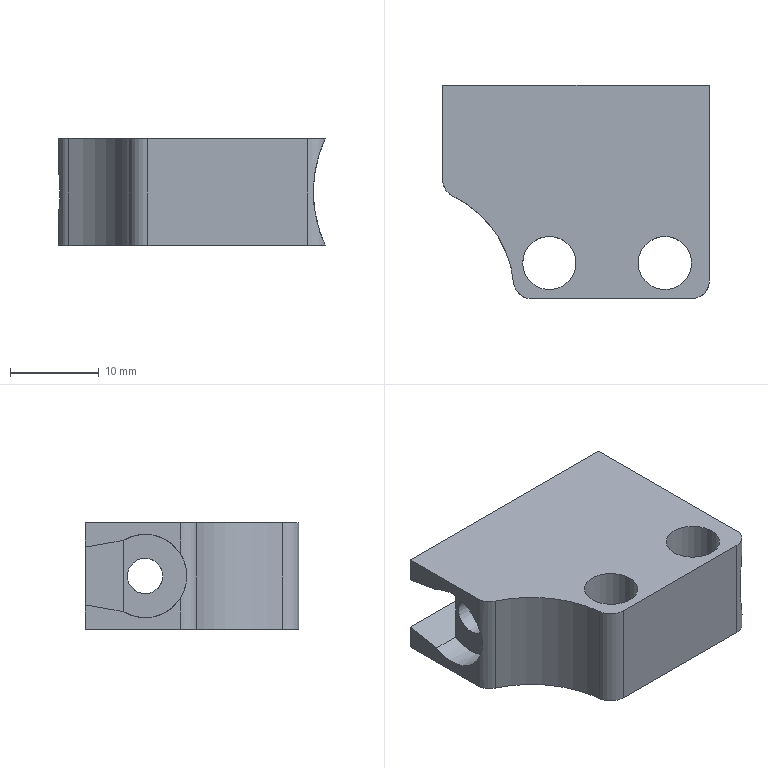Part | NX | features DATUM_CSYS 7, EXTRUDE 7, SKETCH 6, BLEND 1, CPROJ 1 | 1 solid | 20 faces | box 30 x 24 x 12 mm | volume 5622 mm3 | plane 11 | cylinder 9 | commonest cylinder face diameters 4 x4 6 x2 9.4 x1 24 x1 28 x1
STEP:
#1=CARTESIAN_POINT('',(0.,21.08,-6.));
#2=VERTEX_POINT('',#1);
#3=CARTESIAN_POINT('',(0.,21.08,6.));
#4=VERTEX_POINT('',#3);
#5=CARTESIAN_POINT('',(12.649,21.08,0.));
#6=DIRECTION('',(0.,1.,0.));
#7=DIRECTION('',(1.,0.,0.));
#8=AXIS2_PLACEMENT_3D('',#5,#6,#7);
#9=CIRCLE('',#8,14.);
#10=EDGE_CURVE('',#2,#4,#9,.T.);
#11=ORIENTED_EDGE('',*,*,#10,.F.);
#12=CARTESIAN_POINT('',(-30.,21.08,-6.));
#13=VERTEX_POINT('',#12);
#14=CARTESIAN_POINT('',(0.,21.08,-6.));
#15=DIRECTION('',(-1.,0.,0.));
#16=VECTOR('',#15,1000.);
#17=LINE('',#14,#16);
#18=EDGE_CURVE('',#2,#13,#17,.T.);
#19=ORIENTED_EDGE('',*,*,#18,.T.);
#20=CARTESIAN_POINT('',(-30.,21.08,-3.25));
#21=VERTEX_POINT('',#20);
#22=CARTESIAN_POINT('',(-30.,21.08,6.));
#23=DIRECTION('',(0.,0.,-1.));
#24=VECTOR('',#23,1000.);
#25=LINE('',#22,#24);
#26=EDGE_CURVE('',#21,#13,#25,.T.);
#27=ORIENTED_EDGE('',*,*,#26,.F.);
#28=CARTESIAN_POINT('',(-7.,21.08,-3.25));
#29=VERTEX_POINT('',#28);
#30=CARTESIAN_POINT('',(-7.,21.08,-3.25));
#31=DIRECTION('',(-1.,0.,0.));
#32=VECTOR('',#31,1000.);
#33=LINE('',#30,#32);
#34=EDGE_CURVE('',#29,#21,#33,.T.);
#35=ORIENTED_EDGE('',*,*,#34,.F.);
#36=CARTESIAN_POINT('',(-7.,21.08,3.25));
#37=VERTEX_POINT('',#36);
#38=CARTESIAN_POINT('',(-7.,21.08,3.25));
#39=DIRECTION('',(0.,0.,-1.));
#40=VECTOR('',#39,1000.);
#41=LINE('',#38,#40);
#42=EDGE_CURVE('',#37,#29,#41,.T.);
#43=ORIENTED_EDGE('',*,*,#42,.F.);
#44=CARTESIAN_POINT('',(-30.,21.08,3.25));
#45=VERTEX_POINT('',#44);
#46=CARTESIAN_POINT('',(-7.,21.08,3.25));
#47=DIRECTION('',(-1.,0.,0.));
#48=VECTOR('',#47,1000.);
#49=LINE('',#46,#48);
#50=EDGE_CURVE('',#37,#45,#49,.T.);
#51=ORIENTED_EDGE('',*,*,#50,.T.);
#52=CARTESIAN_POINT('',(-30.,21.08,6.));
#53=VERTEX_POINT('',#52);
#54=CARTESIAN_POINT('',(-30.,21.08,6.));
#55=DIRECTION('',(0.,0.,-1.));
#56=VECTOR('',#55,1000.);
#57=LINE('',#54,#56);
#58=EDGE_CURVE('',#53,#45,#57,.T.);
#59=ORIENTED_EDGE('',*,*,#58,.F.);
#60=CARTESIAN_POINT('',(0.,21.08,6.));
#61=DIRECTION('',(-1.,0.,0.));
#62=VECTOR('',#61,1000.);
#63=LINE('',#60,#62);
#64=EDGE_CURVE('',#4,#53,#63,.T.);
#65=ORIENTED_EDGE('',*,*,#64,.F.);
#66=EDGE_LOOP('',(#11,#19,#27,#35,#43,#51,#59,#65));
#67=FACE_BOUND('',#66,.T.);
#68=CARTESIAN_POINT('',(0.,21.08,6.));
#69=DIRECTION('',(0.,-1.,0.));
#70=DIRECTION('',(1.,0.,0.));
#71=AXIS2_PLACEMENT_3D('',#68,#69,#70);
#72=PLANE('',#71);
#73=ADVANCED_FACE('',(#67),#72,.F.);
#74=CARTESIAN_POINT('',(-27.,16.826,4.));
#75=VERTEX_POINT('',#74);
#76=CARTESIAN_POINT('',(-27.,16.826,-4.));
#77=VERTEX_POINT('',#76);
#78=CARTESIAN_POINT('',(-27.,16.826,4.));
#79=DIRECTION('',(0.,0.,-1.));
#80=VECTOR('',#79,1000.);
#81=LINE('',#78,#80);
#82=EDGE_CURVE('',#75,#77,#81,.T.);
#83=ORIENTED_EDGE('',*,*,#82,.F.);
#84=CARTESIAN_POINT('',(-7.,16.826,4.));
#85=VERTEX_POINT('',#84);
#86=CARTESIAN_POINT('',(-7.,16.826,4.));
#87=DIRECTION('',(-1.,0.,0.));
#88=VECTOR('',#87,1000.);
#89=LINE('',#86,#88);
#90=EDGE_CURVE('',#75,#85,#89,.F.);
#91=ORIENTED_EDGE('',*,*,#90,.T.);
#92=CARTESIAN_POINT('',(-7.,16.826,-4.));
#93=VERTEX_POINT('',#92);
#94=CARTESIAN_POINT('',(-7.,16.826,-4.));
#95=DIRECTION('',(0.,0.,1.));
#96=VECTOR('',#95,1000.);
#97=LINE('',#94,#96);
#98=EDGE_CURVE('',#85,#93,#97,.F.);
#99=ORIENTED_EDGE('',*,*,#98,.T.);
#100=CARTESIAN_POINT('',(-7.,16.826,-4.));
#101=DIRECTION('',(-1.,0.,0.));
#102=VECTOR('',#101,1000.);
#103=LINE('',#100,#102);
#104=EDGE_CURVE('',#77,#93,#103,.F.);
#105=ORIENTED_EDGE('',*,*,#104,.F.);
#106=EDGE_LOOP('',(#83,#91,#99,#105));
#107=FACE_BOUND('',#106,.T.);
#108=CARTESIAN_POINT('',(-7.,16.826,0.));
#109=DIRECTION('',(0.,-1.,0.));
#110=DIRECTION('',(1.,0.,0.));
#111=AXIS2_PLACEMENT_3D('',#108,#109,#110);
#112=PLANE('',#111);
#113=ADVANCED_FACE('',(#107),#112,.F.);
#114=CARTESIAN_POINT('',(-30.,10.418,2.561));
#115=VERTEX_POINT('',#114);
#116=CARTESIAN_POINT('',(-30.,16.826,4.));
#117=VERTEX_POINT('',#116);
#118=CARTESIAN_POINT('',(-30.,14.359,0.));
#119=DIRECTION('',(-1.,0.,0.));
#120=DIRECTION('',(0.,0.,1.));
#121=AXIS2_PLACEMENT_3D('',#118,#119,#120);
#122=CIRCLE('',#121,4.7);
#123=EDGE_CURVE('',#115,#117,#122,.T.);
#124=ORIENTED_EDGE('',*,*,#123,.F.);
#125=CARTESIAN_POINT('',(-30.,10.418,6.));
#126=VERTEX_POINT('',#125);
#127=CARTESIAN_POINT('',(-30.,10.418,6.));
#128=DIRECTION('',(0.,0.,-1.));
#129=VECTOR('',#128,1000.);
#130=LINE('',#127,#129);
#131=EDGE_CURVE('',#115,#126,#130,.F.);
#132=ORIENTED_EDGE('',*,*,#131,.T.);
#133=CARTESIAN_POINT('',(-30.,21.08,6.));
#134=DIRECTION('',(0.,-1.,0.));
#135=VECTOR('',#134,1000.);
#136=LINE('',#133,#135);
#137=EDGE_CURVE('',#53,#126,#136,.T.);
#138=ORIENTED_EDGE('',*,*,#137,.F.);
#139=ORIENTED_EDGE('',*,*,#58,.T.);
#140=CARTESIAN_POINT('',(-30.,16.826,4.));
#141=DIRECTION('',(0.,0.9848,-0.1736));
#142=VECTOR('',#141,1000.);
#143=LINE('',#140,#142);
#144=EDGE_CURVE('',#117,#45,#143,.T.);
#145=ORIENTED_EDGE('',*,*,#144,.F.);
#146=EDGE_LOOP('',(#124,#132,#138,#139,#145));
#147=FACE_BOUND('',#146,.T.);
#148=CARTESIAN_POINT('',(-30.,21.08,6.));
#149=DIRECTION('',(1.,0.,0.));
#150=DIRECTION('',(0.,1.,0.));
#151=AXIS2_PLACEMENT_3D('',#148,#149,#150);
#152=PLANE('',#151);
#153=ADVANCED_FACE('',(#147),#152,.F.);
#154=CARTESIAN_POINT('',(-30.,16.826,-4.));
#155=VERTEX_POINT('',#154);
#156=CARTESIAN_POINT('',(-30.,10.418,-2.561));
#157=VERTEX_POINT('',#156);
#158=CARTESIAN_POINT('',(-30.,14.359,0.));
#159=DIRECTION('',(-1.,0.,0.));
#160=DIRECTION('',(0.,0.,1.));
#161=AXIS2_PLACEMENT_3D('',#158,#159,#160);
#162=CIRCLE('',#161,4.7);
#163=EDGE_CURVE('',#155,#157,#162,.T.);
#164=ORIENTED_EDGE('',*,*,#163,.F.);
#165=CARTESIAN_POINT('',(-30.,21.08,-3.25));
#166=DIRECTION('',(0.,-0.9848,-0.1736));
#167=VECTOR('',#166,1000.);
#168=LINE('',#165,#167);
#169=EDGE_CURVE('',#21,#155,#168,.T.);
#170=ORIENTED_EDGE('',*,*,#169,.F.);
#171=ORIENTED_EDGE('',*,*,#26,.T.);
#172=CARTESIAN_POINT('',(-30.,10.418,-6.));
#173=VERTEX_POINT('',#172);
#174=CARTESIAN_POINT('',(-30.,21.08,-6.));
#175=DIRECTION('',(0.,-1.,0.));
#176=VECTOR('',#175,1000.);
#177=LINE('',#174,#176);
#178=EDGE_CURVE('',#13,#173,#177,.T.);
#179=ORIENTED_EDGE('',*,*,#178,.T.);
#180=CARTESIAN_POINT('',(-30.,10.418,6.));
#181=DIRECTION('',(0.,0.,-1.));
#182=VECTOR('',#181,1000.);
#183=LINE('',#180,#182);
#184=EDGE_CURVE('',#173,#157,#183,.F.);
#185=ORIENTED_EDGE('',*,*,#184,.T.);
#186=EDGE_LOOP('',(#164,#170,#171,#179,#185));
#187=FACE_BOUND('',#186,.T.);
#188=CARTESIAN_POINT('',(-30.,21.08,6.));
#189=DIRECTION('',(1.,0.,0.));
#190=DIRECTION('',(0.,1.,0.));
#191=AXIS2_PLACEMENT_3D('',#188,#189,#190);
#192=PLANE('',#191);
#193=ADVANCED_FACE('',(#187),#192,.F.);
#194=CARTESIAN_POINT('',(-28.854,8.609,-6.));
#195=VERTEX_POINT('',#194);
#196=CARTESIAN_POINT('',(-22.034,-1.109,-6.));
#197=VERTEX_POINT('',#196);
#198=CARTESIAN_POINT('',(-33.981,-2.241,-6.));
#199=DIRECTION('',(0.,0.,-1.));
#200=DIRECTION('',(1.,0.,0.));
#201=AXIS2_PLACEMENT_3D('',#198,#199,#200);
#202=CIRCLE('',#201,12.);
#203=EDGE_CURVE('',#195,#197,#202,.T.);
#204=ORIENTED_EDGE('',*,*,#203,.T.);
#205=CARTESIAN_POINT('',(-22.034,-1.109,6.));
#206=VERTEX_POINT('',#205);
#207=CARTESIAN_POINT('',(-22.034,-1.109,6.));
#208=DIRECTION('',(0.,0.,-1.));
#209=VECTOR('',#208,1000.);
#210=LINE('',#207,#209);
#211=EDGE_CURVE('',#197,#206,#210,.F.);
#212=ORIENTED_EDGE('',*,*,#211,.T.);
#213=CARTESIAN_POINT('',(-28.854,8.609,6.));
#214=VERTEX_POINT('',#213);
#215=CARTESIAN_POINT('',(-33.981,-2.241,6.));
#216=DIRECTION('',(0.,0.,-1.));
#217=DIRECTION('',(1.,0.,0.));
#218=AXIS2_PLACEMENT_3D('',#215,#216,#217);
#219=CIRCLE('',#218,12.);
#220=EDGE_CURVE('',#214,#206,#219,.T.);
#221=ORIENTED_EDGE('',*,*,#220,.F.);
#222=CARTESIAN_POINT('',(-28.854,8.609,6.));
#223=DIRECTION('',(0.,0.,-1.));
#224=VECTOR('',#223,1000.);
#225=LINE('',#222,#224);
#226=EDGE_CURVE('',#214,#195,#225,.T.);
#227=ORIENTED_EDGE('',*,*,#226,.T.);
#228=EDGE_LOOP('',(#204,#212,#221,#227));
#229=FACE_BOUND('',#228,.T.);
#230=CARTESIAN_POINT('',(-33.981,-2.241,6.));
#231=DIRECTION('',(0.,0.,-1.));
#232=DIRECTION('',(-1.,0.,0.));
#233=AXIS2_PLACEMENT_3D('',#230,#231,#232);
#234=CYLINDRICAL_SURFACE('',#233,12.);
#235=ADVANCED_FACE('',(#229),#234,.F.);
#236=CARTESIAN_POINT('',(-20.043,-2.92,-6.));
#237=VERTEX_POINT('',#236);
#238=CARTESIAN_POINT('',(-2.,-2.92,-6.));
#239=VERTEX_POINT('',#238);
#240=CARTESIAN_POINT('',(-22.,-2.92,-6.));
#241=DIRECTION('',(1.,0.,0.));
#242=VECTOR('',#241,1000.);
#243=LINE('',#240,#242);
#244=EDGE_CURVE('',#237,#239,#243,.T.);
#245=ORIENTED_EDGE('',*,*,#244,.T.);
#246=CARTESIAN_POINT('',(-2.,-2.92,6.));
#247=VERTEX_POINT('',#246);
#248=CARTESIAN_POINT('',(-2.,-2.92,6.));
#249=DIRECTION('',(0.,0.,-1.));
#250=VECTOR('',#249,1000.);
#251=LINE('',#248,#250);
#252=EDGE_CURVE('',#239,#247,#251,.F.);
#253=ORIENTED_EDGE('',*,*,#252,.T.);
#254=CARTESIAN_POINT('',(-20.043,-2.92,6.));
#255=VERTEX_POINT('',#254);
#256=CARTESIAN_POINT('',(-22.,-2.92,6.));
#257=DIRECTION('',(1.,0.,0.));
#258=VECTOR('',#257,1000.);
#259=LINE('',#256,#258);
#260=EDGE_CURVE('',#255,#247,#259,.T.);
#261=ORIENTED_EDGE('',*,*,#260,.F.);
#262=CARTESIAN_POINT('',(-20.043,-2.92,6.));
#263=DIRECTION('',(0.,0.,-1.));
#264=VECTOR('',#263,1000.);
#265=LINE('',#262,#264);
#266=EDGE_CURVE('',#255,#237,#265,.T.);
#267=ORIENTED_EDGE('',*,*,#266,.T.);
#268=EDGE_LOOP('',(#245,#253,#261,#267));
#269=FACE_BOUND('',#268,.T.);
#270=CARTESIAN_POINT('',(-22.,-2.92,6.));
#271=DIRECTION('',(0.,1.,0.));
#272=DIRECTION('',(0.,0.,1.));
#273=AXIS2_PLACEMENT_3D('',#270,#271,#272);
#274=PLANE('',#273);
#275=ADVANCED_FACE('',(#269),#274,.F.);
#276=CARTESIAN_POINT('',(-2.,1.08,6.));
#277=VERTEX_POINT('',#276);
#278=CARTESIAN_POINT('',(-5.,1.08,6.));
#279=DIRECTION('',(0.,0.,1.));
#280=DIRECTION('',(1.,0.,0.));
#281=AXIS2_PLACEMENT_3D('',#278,#279,#280);
#282=CIRCLE('',#281,3.);
#283=EDGE_CURVE('',#277,#277,#282,.T.);
#284=ORIENTED_EDGE('',*,*,#283,.F.);
#285=EDGE_LOOP('',(#284));
#286=FACE_BOUND('',#285,.T.);
#287=CARTESIAN_POINT('',(-15.,1.08,6.));
#288=VERTEX_POINT('',#287);
#289=CARTESIAN_POINT('',(-18.,1.08,6.));
#290=DIRECTION('',(0.,0.,1.));
#291=DIRECTION('',(1.,0.,0.));
#292=AXIS2_PLACEMENT_3D('',#289,#290,#291);
#293=CIRCLE('',#292,3.);
#294=EDGE_CURVE('',#288,#288,#293,.T.);
#295=ORIENTED_EDGE('',*,*,#294,.F.);
#296=EDGE_LOOP('',(#295));
#297=FACE_BOUND('',#296,.T.);
#298=ORIENTED_EDGE('',*,*,#260,.T.);
#299=CARTESIAN_POINT('',(0.,-0.9202,6.));
#300=VERTEX_POINT('',#299);
#301=CARTESIAN_POINT('',(-2.,-0.9202,6.));
#302=DIRECTION('',(0.,0.,-1.));
#303=DIRECTION('',(-1.,0.,0.));
#304=AXIS2_PLACEMENT_3D('',#301,#302,#303);
#305=CIRCLE('',#304,2.);
#306=EDGE_CURVE('',#247,#300,#305,.F.);
#307=ORIENTED_EDGE('',*,*,#306,.T.);
#308=CARTESIAN_POINT('',(0.,-2.92,6.));
#309=DIRECTION('',(0.,1.,0.));
#310=VECTOR('',#309,1000.);
#311=LINE('',#308,#310);
#312=EDGE_CURVE('',#300,#4,#311,.T.);
#313=ORIENTED_EDGE('',*,*,#312,.T.);
#314=ORIENTED_EDGE('',*,*,#64,.T.);
#315=ORIENTED_EDGE('',*,*,#137,.T.);
#316=CARTESIAN_POINT('',(-28.,10.418,6.));
#317=DIRECTION('',(0.,0.,-1.));
#318=DIRECTION('',(-1.,0.,0.));
#319=AXIS2_PLACEMENT_3D('',#316,#317,#318);
#320=CIRCLE('',#319,2.);
#321=EDGE_CURVE('',#126,#214,#320,.F.);
#322=ORIENTED_EDGE('',*,*,#321,.T.);
#323=ORIENTED_EDGE('',*,*,#220,.T.);
#324=CARTESIAN_POINT('',(-20.043,-0.9202,6.));
#325=DIRECTION('',(0.,0.,-1.));
#326=DIRECTION('',(-1.,0.,0.));
#327=AXIS2_PLACEMENT_3D('',#324,#325,#326);
#328=CIRCLE('',#327,2.);
#329=EDGE_CURVE('',#206,#255,#328,.F.);
#330=ORIENTED_EDGE('',*,*,#329,.T.);
#331=EDGE_LOOP('',(#298,#307,#313,#314,#315,#322,#323,#330));
#332=FACE_BOUND('',#331,.T.);
#333=CARTESIAN_POINT('',(-33.981,-2.241,6.));
#334=DIRECTION('',(0.,0.,-1.));
#335=DIRECTION('',(-1.,0.,0.));
#336=AXIS2_PLACEMENT_3D('',#333,#334,#335);
#337=PLANE('',#336);
#338=ADVANCED_FACE('',(#286,#297,#332),#337,.F.);
#339=CARTESIAN_POINT('',(-8.,1.08,-6.));
#340=VERTEX_POINT('',#339);
#341=CARTESIAN_POINT('',(-5.,1.08,-6.));
#342=DIRECTION('',(0.,0.,-1.));
#343=DIRECTION('',(-1.,0.,0.));
#344=AXIS2_PLACEMENT_3D('',#341,#342,#343);
#345=CIRCLE('',#344,3.);
#346=EDGE_CURVE('',#340,#340,#345,.T.);
#347=ORIENTED_EDGE('',*,*,#346,.F.);
#348=EDGE_LOOP('',(#347));
#349=FACE_BOUND('',#348,.T.);
#350=CARTESIAN_POINT('',(-21.,1.08,-6.));
#351=VERTEX_POINT('',#350);
#352=CARTESIAN_POINT('',(-18.,1.08,-6.));
#353=DIRECTION('',(0.,0.,-1.));
#354=DIRECTION('',(-1.,0.,0.));
#355=AXIS2_PLACEMENT_3D('',#352,#353,#354);
#356=CIRCLE('',#355,3.);
#357=EDGE_CURVE('',#351,#351,#356,.T.);
#358=ORIENTED_EDGE('',*,*,#357,.F.);
#359=EDGE_LOOP('',(#358));
#360=FACE_BOUND('',#359,.T.);
#361=CARTESIAN_POINT('',(0.,-0.9202,-6.));
#362=VERTEX_POINT('',#361);
#363=CARTESIAN_POINT('',(0.,-2.92,-6.));
#364=DIRECTION('',(0.,1.,0.));
#365=VECTOR('',#364,1000.);
#366=LINE('',#363,#365);
#367=EDGE_CURVE('',#362,#2,#366,.T.);
#368=ORIENTED_EDGE('',*,*,#367,.F.);
#369=CARTESIAN_POINT('',(-2.,-0.9202,-6.));
#370=DIRECTION('',(0.,0.,-1.));
#371=DIRECTION('',(-1.,0.,0.));
#372=AXIS2_PLACEMENT_3D('',#369,#370,#371);
#373=CIRCLE('',#372,2.);
#374=EDGE_CURVE('',#362,#239,#373,.T.);
#375=ORIENTED_EDGE('',*,*,#374,.T.);
#376=ORIENTED_EDGE('',*,*,#244,.F.);
#377=CARTESIAN_POINT('',(-20.043,-0.9202,-6.));
#378=DIRECTION('',(0.,0.,-1.));
#379=DIRECTION('',(-1.,0.,0.));
#380=AXIS2_PLACEMENT_3D('',#377,#378,#379);
#381=CIRCLE('',#380,2.);
#382=EDGE_CURVE('',#237,#197,#381,.T.);
#383=ORIENTED_EDGE('',*,*,#382,.T.);
#384=ORIENTED_EDGE('',*,*,#203,.F.);
#385=CARTESIAN_POINT('',(-28.,10.418,-6.));
#386=DIRECTION('',(0.,0.,-1.));
#387=DIRECTION('',(-1.,0.,0.));
#388=AXIS2_PLACEMENT_3D('',#385,#386,#387);
#389=CIRCLE('',#388,2.);
#390=EDGE_CURVE('',#195,#173,#389,.T.);
#391=ORIENTED_EDGE('',*,*,#390,.T.);
#392=ORIENTED_EDGE('',*,*,#178,.F.);
#393=ORIENTED_EDGE('',*,*,#18,.F.);
#394=EDGE_LOOP('',(#368,#375,#376,#383,#384,#391,#392,#393));
#395=FACE_BOUND('',#394,.T.);
#396=CARTESIAN_POINT('',(-33.981,-2.241,-6.));
#397=DIRECTION('',(0.,0.,-1.));
#398=DIRECTION('',(-1.,0.,0.));
#399=AXIS2_PLACEMENT_3D('',#396,#397,#398);
#400=PLANE('',#399);
#401=ADVANCED_FACE('',(#349,#360,#395),#400,.T.);
#402=CARTESIAN_POINT('',(0.,-0.9202,6.));
#403=CARTESIAN_POINT('',(0.,-1.215,6.));
#404=CARTESIAN_POINT('',(-0.139,-1.749,5.71));
#405=CARTESIAN_POINT('',(-0.5326,-2.333,4.77));
#406=CARTESIAN_POINT('',(-0.9643,-2.651,3.417));
#407=CARTESIAN_POINT('',(-1.281,-2.79,1.714));
#408=CARTESIAN_POINT('',(-1.386,-2.823,0.007999));
#409=CARTESIAN_POINT('',(-1.28,-2.79,-1.723));
#410=CARTESIAN_POINT('',(-0.9638,-2.65,-3.419));
#411=CARTESIAN_POINT('',(-0.5302,-2.331,-4.777));
#412=CARTESIAN_POINT('',(-0.1375,-1.745,-5.713));
#413=CARTESIAN_POINT('',(0.,-1.214,-6.));
#414=CARTESIAN_POINT('',(0.,-0.9202,-6.));
#415=B_SPLINE_CURVE_WITH_KNOTS('',3,(#402,#403,#404,#405,#406,#407,#408,#409,#410,#411,#412,#413,#414),.UNSPECIFIED.,.F.,.F.,(4,1,1,1,1,1,1,1,1,1,4),(0.,0.0008713,0.001743,0.003485,0.005228,0.00697,0.008713,0.01046,0.0122,0.01307,0.01394),.UNSPECIFIED.);
#416=EDGE_CURVE('',#300,#362,#415,.T.);
#417=ORIENTED_EDGE('',*,*,#416,.F.);
#418=ORIENTED_EDGE('',*,*,#306,.F.);
#419=ORIENTED_EDGE('',*,*,#252,.F.);
#420=ORIENTED_EDGE('',*,*,#374,.F.);
#421=EDGE_LOOP('',(#417,#418,#419,#420));
#422=FACE_BOUND('',#421,.T.);
#423=CARTESIAN_POINT('',(-2.,-0.9202,6.));
#424=DIRECTION('',(0.,0.,-1.));
#425=DIRECTION('',(-1.,0.,0.));
#426=AXIS2_PLACEMENT_3D('',#423,#424,#425);
#427=CYLINDRICAL_SURFACE('',#426,2.);
#428=ADVANCED_FACE('',(#422),#427,.T.);
#429=ORIENTED_EDGE('',*,*,#329,.F.);
#430=ORIENTED_EDGE('',*,*,#211,.F.);
#431=ORIENTED_EDGE('',*,*,#382,.F.);
#432=ORIENTED_EDGE('',*,*,#266,.F.);
#433=EDGE_LOOP('',(#429,#430,#431,#432));
#434=FACE_BOUND('',#433,.T.);
#435=CARTESIAN_POINT('',(-20.043,-0.9202,6.));
#436=DIRECTION('',(0.,0.,-1.));
#437=DIRECTION('',(-1.,0.,0.));
#438=AXIS2_PLACEMENT_3D('',#435,#436,#437);
#439=CYLINDRICAL_SURFACE('',#438,2.);
#440=ADVANCED_FACE('',(#434),#439,.T.);
#441=CARTESIAN_POINT('',(-30.,10.418,-2.561));
#442=CARTESIAN_POINT('',(-30.,9.92,-1.795));
#443=CARTESIAN_POINT('',(-29.701,9.397,-0.008286));
#444=CARTESIAN_POINT('',(-30.,9.921,1.796));
#445=CARTESIAN_POINT('',(-30.,10.418,2.561));
#446=B_SPLINE_CURVE_WITH_KNOTS('',3,(#441,#442,#443,#444,#445),.UNSPECIFIED.,.F.,.F.,(4,1,4),(0.,0.002701,0.005401),.UNSPECIFIED.);
#447=EDGE_CURVE('',#157,#115,#446,.T.);
#448=ORIENTED_EDGE('',*,*,#447,.F.);
#449=ORIENTED_EDGE('',*,*,#184,.F.);
#450=ORIENTED_EDGE('',*,*,#390,.F.);
#451=ORIENTED_EDGE('',*,*,#226,.F.);
#452=ORIENTED_EDGE('',*,*,#321,.F.);
#453=ORIENTED_EDGE('',*,*,#131,.F.);
#454=EDGE_LOOP('',(#448,#449,#450,#451,#452,#453));
#455=FACE_BOUND('',#454,.T.);
#456=CARTESIAN_POINT('',(-28.,10.418,6.));
#457=DIRECTION('',(0.,0.,-1.));
#458=DIRECTION('',(-1.,0.,0.));
#459=AXIS2_PLACEMENT_3D('',#456,#457,#458);
#460=CYLINDRICAL_SURFACE('',#459,2.);
#461=ADVANCED_FACE('',(#455),#460,.T.);
#462=ORIENTED_EDGE('',*,*,#144,.T.);
#463=ORIENTED_EDGE('',*,*,#50,.F.);
#464=CARTESIAN_POINT('',(-7.,16.826,4.));
#465=DIRECTION('',(0.,0.9848,-0.1736));
#466=VECTOR('',#465,1000.);
#467=LINE('',#464,#466);
#468=EDGE_CURVE('',#37,#85,#467,.F.);
#469=ORIENTED_EDGE('',*,*,#468,.T.);
#470=ORIENTED_EDGE('',*,*,#90,.F.);
#471=CARTESIAN_POINT('',(-7.,16.826,4.));
#472=DIRECTION('',(-1.,0.,0.));
#473=VECTOR('',#472,1000.);
#474=LINE('',#471,#473);
#475=EDGE_CURVE('',#117,#75,#474,.F.);
#476=ORIENTED_EDGE('',*,*,#475,.F.);
#477=EDGE_LOOP('',(#462,#463,#469,#470,#476));
#478=FACE_BOUND('',#477,.T.);
#479=CARTESIAN_POINT('',(-7.,16.826,4.));
#480=DIRECTION('',(0.,0.1736,0.9848));
#481=DIRECTION('',(0.,-0.9848,0.1736));
#482=AXIS2_PLACEMENT_3D('',#479,#480,#481);
#483=PLANE('',#482);
#484=ADVANCED_FACE('',(#478),#483,.F.);
#485=ORIENTED_EDGE('',*,*,#169,.T.);
#486=CARTESIAN_POINT('',(-7.,16.826,-4.));
#487=DIRECTION('',(-1.,0.,0.));
#488=VECTOR('',#487,1000.);
#489=LINE('',#486,#488);
#490=EDGE_CURVE('',#155,#77,#489,.F.);
#491=ORIENTED_EDGE('',*,*,#490,.T.);
#492=ORIENTED_EDGE('',*,*,#104,.T.);
#493=CARTESIAN_POINT('',(-7.,21.08,-3.25));
#494=DIRECTION('',(0.,-0.9848,-0.1736));
#495=VECTOR('',#494,1000.);
#496=LINE('',#493,#495);
#497=EDGE_CURVE('',#93,#29,#496,.F.);
#498=ORIENTED_EDGE('',*,*,#497,.T.);
#499=ORIENTED_EDGE('',*,*,#34,.T.);
#500=EDGE_LOOP('',(#485,#491,#492,#498,#499));
#501=FACE_BOUND('',#500,.T.);
#502=CARTESIAN_POINT('',(-7.,21.08,-3.25));
#503=DIRECTION('',(0.,0.1736,-0.9848));
#504=DIRECTION('',(0.,0.9848,0.1736));
#505=AXIS2_PLACEMENT_3D('',#502,#503,#504);
#506=PLANE('',#505);
#507=ADVANCED_FACE('',(#501),#506,.F.);
#508=ORIENTED_EDGE('',*,*,#98,.F.);
#509=ORIENTED_EDGE('',*,*,#468,.F.);
#510=ORIENTED_EDGE('',*,*,#42,.T.);
#511=ORIENTED_EDGE('',*,*,#497,.F.);
#512=EDGE_LOOP('',(#508,#509,#510,#511));
#513=FACE_BOUND('',#512,.T.);
#514=CARTESIAN_POINT('',(-7.,0.,0.));
#515=DIRECTION('',(-1.,0.,0.));
#516=DIRECTION('',(0.,0.,1.));
#517=AXIS2_PLACEMENT_3D('',#514,#515,#516);
#518=PLANE('',#517);
#519=ADVANCED_FACE('',(#513),#518,.T.);
#520=ORIENTED_EDGE('',*,*,#447,.T.);
#521=ORIENTED_EDGE('',*,*,#123,.T.);
#522=ORIENTED_EDGE('',*,*,#475,.T.);
#523=CARTESIAN_POINT('',(-27.,14.359,0.));
#524=DIRECTION('',(-1.,0.,0.));
#525=DIRECTION('',(0.,0.,1.));
#526=AXIS2_PLACEMENT_3D('',#523,#524,#525);
#527=CIRCLE('',#526,4.7);
#528=EDGE_CURVE('',#75,#77,#527,.F.);
#529=ORIENTED_EDGE('',*,*,#528,.T.);
#530=ORIENTED_EDGE('',*,*,#490,.F.);
#531=ORIENTED_EDGE('',*,*,#163,.T.);
#532=EDGE_LOOP('',(#520,#521,#522,#529,#530,#531));
#533=FACE_BOUND('',#532,.T.);
#534=CARTESIAN_POINT('',(-27.,14.359,0.));
#535=DIRECTION('',(-1.,0.,0.));
#536=DIRECTION('',(0.,-1.,0.));
#537=AXIS2_PLACEMENT_3D('',#534,#535,#536);
#538=CYLINDRICAL_SURFACE('',#537,4.7);
#539=ADVANCED_FACE('',(#533),#538,.F.);
#540=CARTESIAN_POINT('',(-27.,14.359,2.));
#541=VERTEX_POINT('',#540);
#542=CARTESIAN_POINT('',(-27.,14.359,0.));
#543=DIRECTION('',(-1.,0.,0.));
#544=DIRECTION('',(0.,0.,1.));
#545=AXIS2_PLACEMENT_3D('',#542,#543,#544);
#546=CIRCLE('',#545,2.);
#547=EDGE_CURVE('',#541,#541,#546,.T.);
#548=ORIENTED_EDGE('',*,*,#547,.F.);
#549=EDGE_LOOP('',(#548));
#550=FACE_BOUND('',#549,.T.);
#551=ORIENTED_EDGE('',*,*,#528,.F.);
#552=ORIENTED_EDGE('',*,*,#82,.T.);
#553=EDGE_LOOP('',(#551,#552));
#554=FACE_BOUND('',#553,.T.);
#555=CARTESIAN_POINT('',(-27.,14.359,0.));
#556=DIRECTION('',(-1.,0.,0.));
#557=DIRECTION('',(0.,-1.,0.));
#558=AXIS2_PLACEMENT_3D('',#555,#556,#557);
#559=PLANE('',#558);
#560=ADVANCED_FACE('',(#550,#554),#559,.T.);
#561=CARTESIAN_POINT('',(-1.351,12.359,0.));
#562=VERTEX_POINT('',#561);
#563=CARTESIAN_POINT('',(-1.279,12.793,1.569));
#564=CARTESIAN_POINT('',(-1.387,12.142,-0.0003812));
#565=CARTESIAN_POINT('',(-1.279,12.792,-1.567));
#566=CARTESIAN_POINT('',(-1.171,14.357,-2.216));
#567=CARTESIAN_POINT('',(-1.279,15.926,-1.568));
#568=CARTESIAN_POINT('',(-1.387,16.575,-0.000506));
#569=CARTESIAN_POINT('',(-1.28,15.927,1.565));
#570=CARTESIAN_POINT('',(-1.171,14.36,2.216));
#571=CARTESIAN_POINT('',(-1.279,12.793,1.569));
#572=CARTESIAN_POINT('',(-1.387,12.142,-0.0003812));
#573=CARTESIAN_POINT('',(-1.279,12.792,-1.567));
#574=B_SPLINE_CURVE_WITH_KNOTS('',3,(#563,#564,#565,#566,#567,#568,#569,#570,#571,#572,#573),.UNSPECIFIED.,.T.,.F.,(1,1,1,1,1,1,1,1,1,1,1,1,1,1,1),(-0.004695,-0.00313,-0.001565,0.,0.001565,0.00313,0.004695,0.00626,0.007825,0.00939,0.01096,0.01252,0.01409,0.01565,0.01722),.UNSPECIFIED.);
#575=EDGE_CURVE('',#562,#562,#574,.T.);
#576=ORIENTED_EDGE('',*,*,#575,.T.);
#577=EDGE_LOOP('',(#576));
#578=FACE_BOUND('',#577,.T.);
#579=ORIENTED_EDGE('',*,*,#547,.T.);
#580=EDGE_LOOP('',(#579));
#581=FACE_BOUND('',#580,.T.);
#582=CARTESIAN_POINT('',(54973.,14.359,0.));
#583=DIRECTION('',(-1.,0.,0.));
#584=DIRECTION('',(0.,-1.,0.));
#585=AXIS2_PLACEMENT_3D('',#582,#583,#584);
#586=CYLINDRICAL_SURFACE('',#585,2.);
#587=ADVANCED_FACE('',(#578,#581),#586,.F.);
#588=ORIENTED_EDGE('',*,*,#357,.T.);
#589=EDGE_LOOP('',(#588));
#590=FACE_BOUND('',#589,.T.);
#591=ORIENTED_EDGE('',*,*,#294,.T.);
#592=EDGE_LOOP('',(#591));
#593=FACE_BOUND('',#592,.T.);
#594=CARTESIAN_POINT('',(-18.,1.08,-54994.));
#595=DIRECTION('',(0.,0.,1.));
#596=DIRECTION('',(1.,0.,0.));
#597=AXIS2_PLACEMENT_3D('',#594,#595,#596);
#598=CYLINDRICAL_SURFACE('',#597,3.);
#599=ADVANCED_FACE('',(#590,#593),#598,.F.);
#600=ORIENTED_EDGE('',*,*,#346,.T.);
#601=EDGE_LOOP('',(#600));
#602=FACE_BOUND('',#601,.T.);
#603=ORIENTED_EDGE('',*,*,#283,.T.);
#604=EDGE_LOOP('',(#603));
#605=FACE_BOUND('',#604,.T.);
#606=CARTESIAN_POINT('',(-5.,1.08,-54994.));
#607=DIRECTION('',(0.,0.,1.));
#608=DIRECTION('',(1.,0.,0.));
#609=AXIS2_PLACEMENT_3D('',#606,#607,#608);
#610=CYLINDRICAL_SURFACE('',#609,3.);
#611=ADVANCED_FACE('',(#602,#605),#610,.F.);
#612=ORIENTED_EDGE('',*,*,#416,.T.);
#613=ORIENTED_EDGE('',*,*,#367,.T.);
#614=ORIENTED_EDGE('',*,*,#10,.T.);
#615=ORIENTED_EDGE('',*,*,#312,.F.);
#616=EDGE_LOOP('',(#612,#613,#614,#615));
#617=FACE_BOUND('',#616,.T.);
#618=ORIENTED_EDGE('',*,*,#575,.F.);
#619=EDGE_LOOP('',(#618));
#620=FACE_BOUND('',#619,.T.);
#621=CARTESIAN_POINT('',(12.649,-54978.92,0.));
#622=DIRECTION('',(0.,1.,0.));
#623=DIRECTION('',(-1.,0.,0.));
#624=AXIS2_PLACEMENT_3D('',#621,#622,#623);
#625=CYLINDRICAL_SURFACE('',#624,14.);
#626=ADVANCED_FACE('',(#617,#620),#625,.F.);
#627=CLOSED_SHELL('',(#73,#113,#153,#193,#235,#275,#338,#401,#428,#440,#461,#484,#507,#519,#539,#560,#587,#599,#611,#626));
#628=MANIFOLD_SOLID_BREP('',#627);
#629=(LENGTH_UNIT()NAMED_UNIT(*)SI_UNIT(.MILLI.,.METRE.));
#630=UNCERTAINTY_MEASURE_WITH_UNIT(LENGTH_MEASURE(0.0508),#629,'','');
#631=(NAMED_UNIT(*)PLANE_ANGLE_UNIT()SI_UNIT($,.RADIAN.));
#632=(NAMED_UNIT(*)SI_UNIT($,.STERADIAN.)SOLID_ANGLE_UNIT());
#633=(GEOMETRIC_REPRESENTATION_CONTEXT(3)GLOBAL_UNCERTAINTY_ASSIGNED_CONTEXT((#630))GLOBAL_UNIT_ASSIGNED_CONTEXT((#629,#631,#632))REPRESENTATION_CONTEXT('',''));
#634=ADVANCED_BREP_SHAPE_REPRESENTATION('',(#628),#633);